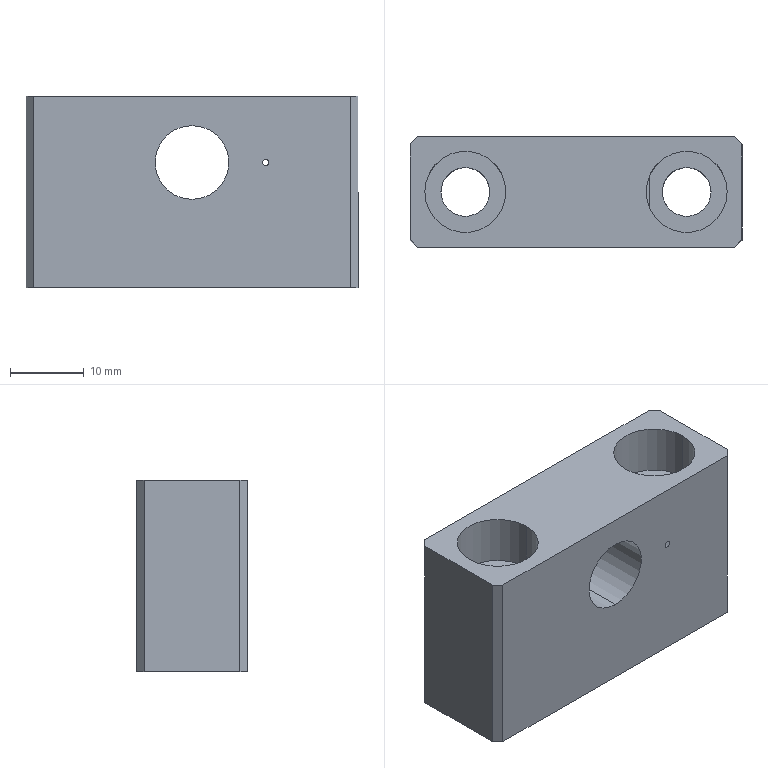Part | SolidWorks | features HoleWzd 3, Chamfer 1, Cut 1, Extrusion 1 | 1 solid | 34 faces | box 45 x 15 x 26 mm | volume 12916 mm3 | cylinder 16 | plane 12 | cone 6 | commonest cylinder face diameters 6 x4 6.6 x4 11 x4 4.2 x2 10 x2
STEP:
#1=CARTESIAN_POINT('',(10.,1.,1.9));
#2=VERTEX_POINT('',#1);
#3=CARTESIAN_POINT('',(10.,1.,6.1));
#4=VERTEX_POINT('',#3);
#5=CARTESIAN_POINT('',(10.,1.,4.));
#6=DIRECTION('',(0.,1.,0.));
#7=DIRECTION('',(0.,0.,1.));
#8=AXIS2_PLACEMENT_3D('',#5,#6,#7);
#9=CIRCLE('',#8,2.1);
#10=EDGE_CURVE('',#2,#4,#9,.T.);
#11=ORIENTED_EDGE('',*,*,#10,.F.);
#12=CARTESIAN_POINT('',(10.,15.,1.9));
#13=VERTEX_POINT('',#12);
#14=CARTESIAN_POINT('',(10.,15.,1.9));
#15=DIRECTION('',(0.,1.,0.));
#16=VECTOR('',#15,1000.);
#17=LINE('',#14,#16);
#18=EDGE_CURVE('',#2,#13,#17,.T.);
#19=ORIENTED_EDGE('',*,*,#18,.T.);
#20=CARTESIAN_POINT('',(10.,15.,6.1));
#21=VERTEX_POINT('',#20);
#22=CARTESIAN_POINT('',(10.,15.,4.));
#23=DIRECTION('',(0.,1.,0.));
#24=DIRECTION('',(0.,0.,1.));
#25=AXIS2_PLACEMENT_3D('',#22,#23,#24);
#26=CIRCLE('',#25,2.1);
#27=EDGE_CURVE('',#13,#21,#26,.T.);
#28=ORIENTED_EDGE('',*,*,#27,.T.);
#29=CARTESIAN_POINT('',(10.,15.,6.1));
#30=DIRECTION('',(0.,1.,0.));
#31=VECTOR('',#30,1000.);
#32=LINE('',#29,#31);
#33=EDGE_CURVE('',#4,#21,#32,.T.);
#34=ORIENTED_EDGE('',*,*,#33,.F.);
#35=EDGE_LOOP('',(#11,#19,#28,#34));
#36=FACE_OUTER_BOUND('',#35,.T.);
#37=CARTESIAN_POINT('',(10.,15.,4.));
#38=DIRECTION('',(0.,1.,0.));
#39=DIRECTION('',(0.,0.,1.));
#40=AXIS2_PLACEMENT_3D('',#37,#38,#39);
#41=CYLINDRICAL_SURFACE('',#40,2.1);
#42=ADVANCED_FACE('',(#36),#41,.F.);
#43=CARTESIAN_POINT('',(10.,0.,3.564));
#44=VERTEX_POINT('',#43);
#45=CARTESIAN_POINT('',(10.,0.,4.436));
#46=VERTEX_POINT('',#45);
#47=CARTESIAN_POINT('',(10.,0.,4.));
#48=DIRECTION('',(0.,1.,0.));
#49=DIRECTION('',(0.,0.,1.));
#50=AXIS2_PLACEMENT_3D('',#47,#48,#49);
#51=CIRCLE('',#50,0.4357);
#52=EDGE_CURVE('',#44,#46,#51,.T.);
#53=ORIENTED_EDGE('',*,*,#52,.F.);
#54=CARTESIAN_POINT('',(10.,1.,1.9));
#55=DIRECTION('',(0.,0.515,-0.8572));
#56=VECTOR('',#55,1000.);
#57=LINE('',#54,#56);
#58=EDGE_CURVE('',#44,#2,#57,.T.);
#59=ORIENTED_EDGE('',*,*,#58,.T.);
#60=ORIENTED_EDGE('',*,*,#10,.T.);
#61=CARTESIAN_POINT('',(10.,1.,6.1));
#62=DIRECTION('',(0.,0.515,0.8572));
#63=VECTOR('',#62,1000.);
#64=LINE('',#61,#63);
#65=EDGE_CURVE('',#46,#4,#64,.T.);
#66=ORIENTED_EDGE('',*,*,#65,.F.);
#67=EDGE_LOOP('',(#53,#59,#60,#66));
#68=FACE_OUTER_BOUND('',#67,.T.);
#69=CARTESIAN_POINT('',(10.,1.,4.));
#70=DIRECTION('',(0.,1.,0.));
#71=DIRECTION('',(0.,0.,1.));
#72=AXIS2_PLACEMENT_3D('',#69,#70,#71);
#73=CONICAL_SURFACE('',#72,2.1,1.03);
#74=ADVANCED_FACE('',(#68),#73,.F.);
#75=CARTESIAN_POINT('',(9.5,7.5,6.2));
#76=VERTEX_POINT('',#75);
#77=CARTESIAN_POINT('',(20.5,7.5,6.2));
#78=VERTEX_POINT('',#77);
#79=CARTESIAN_POINT('',(15.,7.5,6.2));
#80=DIRECTION('',(0.,0.,1.));
#81=DIRECTION('',(1.,0.,0.));
#82=AXIS2_PLACEMENT_3D('',#79,#80,#81);
#83=CIRCLE('',#82,5.5);
#84=EDGE_CURVE('',#76,#78,#83,.T.);
#85=ORIENTED_EDGE('',*,*,#84,.F.);
#86=CARTESIAN_POINT('',(9.5,7.5,13.));
#87=VERTEX_POINT('',#86);
#88=CARTESIAN_POINT('',(9.5,7.5,13.));
#89=DIRECTION('',(0.,0.,1.));
#90=VECTOR('',#89,1000.);
#91=LINE('',#88,#90);
#92=EDGE_CURVE('',#76,#87,#91,.T.);
#93=ORIENTED_EDGE('',*,*,#92,.T.);
#94=CARTESIAN_POINT('',(20.5,7.5,13.));
#95=VERTEX_POINT('',#94);
#96=CARTESIAN_POINT('',(15.,7.5,13.));
#97=DIRECTION('',(0.,0.,1.));
#98=DIRECTION('',(1.,0.,0.));
#99=AXIS2_PLACEMENT_3D('',#96,#97,#98);
#100=CIRCLE('',#99,5.5);
#101=EDGE_CURVE('',#87,#95,#100,.T.);
#102=ORIENTED_EDGE('',*,*,#101,.T.);
#103=CARTESIAN_POINT('',(20.5,7.5,13.));
#104=DIRECTION('',(0.,0.,1.));
#105=VECTOR('',#104,1000.);
#106=LINE('',#103,#105);
#107=EDGE_CURVE('',#78,#95,#106,.T.);
#108=ORIENTED_EDGE('',*,*,#107,.F.);
#109=EDGE_LOOP('',(#85,#93,#102,#108));
#110=FACE_OUTER_BOUND('',#109,.T.);
#111=CARTESIAN_POINT('',(15.,7.5,13.));
#112=DIRECTION('',(0.,0.,1.));
#113=DIRECTION('',(1.,0.,0.));
#114=AXIS2_PLACEMENT_3D('',#111,#112,#113);
#115=CYLINDRICAL_SURFACE('',#114,5.5);
#116=ADVANCED_FACE('',(#110),#115,.F.);
#117=CARTESIAN_POINT('',(11.7,7.5,-13.));
#118=VERTEX_POINT('',#117);
#119=CARTESIAN_POINT('',(18.3,7.5,-13.));
#120=VERTEX_POINT('',#119);
#121=CARTESIAN_POINT('',(15.,7.5,-13.));
#122=DIRECTION('',(0.,0.,1.));
#123=DIRECTION('',(1.,0.,0.));
#124=AXIS2_PLACEMENT_3D('',#121,#122,#123);
#125=CIRCLE('',#124,3.3);
#126=EDGE_CURVE('',#118,#120,#125,.T.);
#127=ORIENTED_EDGE('',*,*,#126,.F.);
#128=CARTESIAN_POINT('',(11.7,7.5,2.767));
#129=VERTEX_POINT('',#128);
#130=CARTESIAN_POINT('',(11.7,7.5,13.));
#131=DIRECTION('',(0.,0.,1.));
#132=VECTOR('',#131,1000.);
#133=LINE('',#130,#132);
#134=EDGE_CURVE('',#118,#129,#133,.T.);
#135=ORIENTED_EDGE('',*,*,#134,.T.);
#136=CARTESIAN_POINT('',(11.7,7.5,5.233));
#137=VERTEX_POINT('',#136);
#138=CARTESIAN_POINT('',(11.7,7.5,2.767));
#139=CARTESIAN_POINT('',(11.7,7.309,2.767));
#140=CARTESIAN_POINT('',(11.716,7.122,2.789));
#141=CARTESIAN_POINT('',(11.779,6.758,2.883));
#142=CARTESIAN_POINT('',(11.824,6.589,2.954));
#143=CARTESIAN_POINT('',(11.902,6.361,3.108));
#144=CARTESIAN_POINT('',(11.929,6.29,3.167));
#145=CARTESIAN_POINT('',(11.981,6.166,3.3));
#146=CARTESIAN_POINT('',(12.006,6.11,3.375));
#147=CARTESIAN_POINT('',(12.071,5.976,3.617));
#148=CARTESIAN_POINT('',(12.1,5.926,3.805));
#149=CARTESIAN_POINT('',(12.1,5.924,4.184));
#150=CARTESIAN_POINT('',(12.073,5.973,4.376));
#151=CARTESIAN_POINT('',(11.987,6.151,4.701));
#152=CARTESIAN_POINT('',(11.93,6.279,4.836));
#153=CARTESIAN_POINT('',(11.826,6.583,5.044));
#154=CARTESIAN_POINT('',(11.78,6.756,5.116));
#155=CARTESIAN_POINT('',(11.717,7.12,5.211));
#156=CARTESIAN_POINT('',(11.7,7.31,5.233));
#157=CARTESIAN_POINT('',(11.7,7.5,5.233));
#158=B_SPLINE_CURVE_WITH_KNOTS('',3,(#138,#139,#140,#141,#142,#143,#144,#145,#146,#147,#148,#149,#150,#151,#152,#153,#154,#155,#156,#157),.UNSPECIFIED.,.F.,.F.,(4,2,2,2,2,2,2,2,2,4),(0.,0.0005661,0.001132,0.001415,0.001698,0.002264,0.002831,0.003397,0.003963,0.004529),.UNSPECIFIED.);
#159=EDGE_CURVE('',#129,#137,#158,.T.);
#160=ORIENTED_EDGE('',*,*,#159,.T.);
#161=CARTESIAN_POINT('',(11.7,7.5,6.2));
#162=VERTEX_POINT('',#161);
#163=CARTESIAN_POINT('',(11.7,7.5,13.));
#164=DIRECTION('',(0.,0.,1.));
#165=VECTOR('',#164,1000.);
#166=LINE('',#163,#165);
#167=EDGE_CURVE('',#137,#162,#166,.T.);
#168=ORIENTED_EDGE('',*,*,#167,.T.);
#169=CARTESIAN_POINT('',(18.3,7.5,6.2));
#170=VERTEX_POINT('',#169);
#171=CARTESIAN_POINT('',(15.,7.5,6.2));
#172=DIRECTION('',(0.,0.,1.));
#173=DIRECTION('',(1.,0.,0.));
#174=AXIS2_PLACEMENT_3D('',#171,#172,#173);
#175=CIRCLE('',#174,3.3);
#176=EDGE_CURVE('',#162,#170,#175,.T.);
#177=ORIENTED_EDGE('',*,*,#176,.T.);
#178=CARTESIAN_POINT('',(18.3,7.5,13.));
#179=DIRECTION('',(0.,0.,1.));
#180=VECTOR('',#179,1000.);
#181=LINE('',#178,#180);
#182=EDGE_CURVE('',#120,#170,#181,.T.);
#183=ORIENTED_EDGE('',*,*,#182,.F.);
#184=EDGE_LOOP('',(#127,#135,#160,#168,#177,#183));
#185=FACE_OUTER_BOUND('',#184,.T.);
#186=CARTESIAN_POINT('',(15.,7.5,13.));
#187=DIRECTION('',(0.,0.,1.));
#188=DIRECTION('',(1.,0.,0.));
#189=AXIS2_PLACEMENT_3D('',#186,#187,#188);
#190=CYLINDRICAL_SURFACE('',#189,3.3);
#191=ADVANCED_FACE('',(#185),#190,.F.);
#192=CARTESIAN_POINT('',(-20.5,7.5,6.2));
#193=VERTEX_POINT('',#192);
#194=CARTESIAN_POINT('',(-9.5,7.5,6.2));
#195=VERTEX_POINT('',#194);
#196=CARTESIAN_POINT('',(-15.,7.5,6.2));
#197=DIRECTION('',(0.,0.,1.));
#198=DIRECTION('',(1.,0.,0.));
#199=AXIS2_PLACEMENT_3D('',#196,#197,#198);
#200=CIRCLE('',#199,5.5);
#201=EDGE_CURVE('',#193,#195,#200,.T.);
#202=ORIENTED_EDGE('',*,*,#201,.F.);
#203=CARTESIAN_POINT('',(-20.5,7.5,13.));
#204=VERTEX_POINT('',#203);
#205=CARTESIAN_POINT('',(-20.5,7.5,13.));
#206=DIRECTION('',(0.,0.,1.));
#207=VECTOR('',#206,1000.);
#208=LINE('',#205,#207);
#209=EDGE_CURVE('',#193,#204,#208,.T.);
#210=ORIENTED_EDGE('',*,*,#209,.T.);
#211=CARTESIAN_POINT('',(-9.5,7.5,13.));
#212=VERTEX_POINT('',#211);
#213=CARTESIAN_POINT('',(-15.,7.5,13.));
#214=DIRECTION('',(0.,0.,1.));
#215=DIRECTION('',(1.,0.,0.));
#216=AXIS2_PLACEMENT_3D('',#213,#214,#215);
#217=CIRCLE('',#216,5.5);
#218=EDGE_CURVE('',#204,#212,#217,.T.);
#219=ORIENTED_EDGE('',*,*,#218,.T.);
#220=CARTESIAN_POINT('',(-9.5,7.5,13.));
#221=DIRECTION('',(0.,0.,1.));
#222=VECTOR('',#221,1000.);
#223=LINE('',#220,#222);
#224=EDGE_CURVE('',#195,#212,#223,.T.);
#225=ORIENTED_EDGE('',*,*,#224,.F.);
#226=EDGE_LOOP('',(#202,#210,#219,#225));
#227=FACE_OUTER_BOUND('',#226,.T.);
#228=CARTESIAN_POINT('',(-15.,7.5,13.));
#229=DIRECTION('',(0.,0.,1.));
#230=DIRECTION('',(1.,0.,0.));
#231=AXIS2_PLACEMENT_3D('',#228,#229,#230);
#232=CYLINDRICAL_SURFACE('',#231,5.5);
#233=ADVANCED_FACE('',(#227),#232,.F.);
#234=CARTESIAN_POINT('',(-18.3,7.5,-13.));
#235=VERTEX_POINT('',#234);
#236=CARTESIAN_POINT('',(-11.7,7.5,-13.));
#237=VERTEX_POINT('',#236);
#238=CARTESIAN_POINT('',(-15.,7.5,-13.));
#239=DIRECTION('',(0.,0.,1.));
#240=DIRECTION('',(1.,0.,0.));
#241=AXIS2_PLACEMENT_3D('',#238,#239,#240);
#242=CIRCLE('',#241,3.3);
#243=EDGE_CURVE('',#235,#237,#242,.T.);
#244=ORIENTED_EDGE('',*,*,#243,.F.);
#245=CARTESIAN_POINT('',(-18.3,7.5,6.2));
#246=VERTEX_POINT('',#245);
#247=CARTESIAN_POINT('',(-18.3,7.5,13.));
#248=DIRECTION('',(0.,0.,1.));
#249=VECTOR('',#248,1000.);
#250=LINE('',#247,#249);
#251=EDGE_CURVE('',#235,#246,#250,.T.);
#252=ORIENTED_EDGE('',*,*,#251,.T.);
#253=CARTESIAN_POINT('',(-11.7,7.5,6.2));
#254=VERTEX_POINT('',#253);
#255=CARTESIAN_POINT('',(-15.,7.5,6.2));
#256=DIRECTION('',(0.,0.,1.));
#257=DIRECTION('',(1.,0.,0.));
#258=AXIS2_PLACEMENT_3D('',#255,#256,#257);
#259=CIRCLE('',#258,3.3);
#260=EDGE_CURVE('',#246,#254,#259,.T.);
#261=ORIENTED_EDGE('',*,*,#260,.T.);
#262=CARTESIAN_POINT('',(-11.7,7.5,13.));
#263=DIRECTION('',(0.,0.,1.));
#264=VECTOR('',#263,1000.);
#265=LINE('',#262,#264);
#266=EDGE_CURVE('',#237,#254,#265,.T.);
#267=ORIENTED_EDGE('',*,*,#266,.F.);
#268=EDGE_LOOP('',(#244,#252,#261,#267));
#269=FACE_OUTER_BOUND('',#268,.T.);
#270=CARTESIAN_POINT('',(-15.,7.5,13.));
#271=DIRECTION('',(0.,0.,1.));
#272=DIRECTION('',(1.,0.,0.));
#273=AXIS2_PLACEMENT_3D('',#270,#271,#272);
#274=CYLINDRICAL_SURFACE('',#273,3.3);
#275=ADVANCED_FACE('',(#269),#274,.F.);
#276=CARTESIAN_POINT('',(-2.,7.5,-3.));
#277=VERTEX_POINT('',#276);
#278=CARTESIAN_POINT('',(-8.,7.5,-3.));
#279=VERTEX_POINT('',#278);
#280=CARTESIAN_POINT('',(-5.,7.5,-3.));
#281=DIRECTION('',(0.,0.,-1.));
#282=DIRECTION('',(-1.,0.,0.));
#283=AXIS2_PLACEMENT_3D('',#280,#281,#282);
#284=CIRCLE('',#283,3.);
#285=EDGE_CURVE('',#277,#279,#284,.T.);
#286=ORIENTED_EDGE('',*,*,#285,.F.);
#287=CARTESIAN_POINT('',(-2.,7.5,-13.));
#288=VERTEX_POINT('',#287);
#289=CARTESIAN_POINT('',(-2.,7.5,-13.));
#290=DIRECTION('',(0.,0.,-1.));
#291=VECTOR('',#290,1000.);
#292=LINE('',#289,#291);
#293=EDGE_CURVE('',#277,#288,#292,.T.);
#294=ORIENTED_EDGE('',*,*,#293,.T.);
#295=CARTESIAN_POINT('',(-8.,7.5,-13.));
#296=VERTEX_POINT('',#295);
#297=CARTESIAN_POINT('',(-5.,7.5,-13.));
#298=DIRECTION('',(0.,0.,-1.));
#299=DIRECTION('',(-1.,0.,0.));
#300=AXIS2_PLACEMENT_3D('',#297,#298,#299);
#301=CIRCLE('',#300,3.);
#302=EDGE_CURVE('',#288,#296,#301,.T.);
#303=ORIENTED_EDGE('',*,*,#302,.T.);
#304=CARTESIAN_POINT('',(-8.,7.5,-13.));
#305=DIRECTION('',(0.,0.,-1.));
#306=VECTOR('',#305,1000.);
#307=LINE('',#304,#306);
#308=EDGE_CURVE('',#279,#296,#307,.T.);
#309=ORIENTED_EDGE('',*,*,#308,.F.);
#310=EDGE_LOOP('',(#286,#294,#303,#309));
#311=FACE_OUTER_BOUND('',#310,.T.);
#312=CARTESIAN_POINT('',(-5.,7.5,-13.));
#313=DIRECTION('',(0.,0.,-1.));
#314=DIRECTION('',(-1.,0.,0.));
#315=AXIS2_PLACEMENT_3D('',#312,#313,#314);
#316=CYLINDRICAL_SURFACE('',#315,3.);
#317=ADVANCED_FACE('',(#311),#316,.F.);
#318=CARTESIAN_POINT('',(-5.,7.5,-1.197));
#319=VERTEX_POINT('',#318);
#320=CARTESIAN_POINT('',(-8.,7.5,-3.));
#321=DIRECTION('',(-0.8572,0.,-0.515));
#322=VECTOR('',#321,1000.);
#323=LINE('',#320,#322);
#324=EDGE_CURVE('',#319,#279,#323,.T.);
#325=ORIENTED_EDGE('',*,*,#324,.F.);
#326=CARTESIAN_POINT('',(-2.,7.5,-3.));
#327=DIRECTION('',(0.8572,0.,-0.515));
#328=VECTOR('',#327,1000.);
#329=LINE('',#326,#328);
#330=EDGE_CURVE('',#319,#277,#329,.T.);
#331=ORIENTED_EDGE('',*,*,#330,.T.);
#332=ORIENTED_EDGE('',*,*,#285,.T.);
#333=EDGE_LOOP('',(#325,#331,#332));
#334=FACE_OUTER_BOUND('',#333,.T.);
#335=CARTESIAN_POINT('',(-5.,7.5,-3.));
#336=DIRECTION('',(0.,0.,-1.));
#337=DIRECTION('',(-1.,0.,0.));
#338=AXIS2_PLACEMENT_3D('',#335,#336,#337);
#339=CONICAL_SURFACE('',#338,3.,1.03);
#340=ADVANCED_FACE('',(#334),#339,.F.);
#341=CARTESIAN_POINT('',(8.,7.5,-3.));
#342=VERTEX_POINT('',#341);
#343=CARTESIAN_POINT('',(2.,7.5,-3.));
#344=VERTEX_POINT('',#343);
#345=CARTESIAN_POINT('',(5.,7.5,-3.));
#346=DIRECTION('',(0.,0.,-1.));
#347=DIRECTION('',(-1.,0.,0.));
#348=AXIS2_PLACEMENT_3D('',#345,#346,#347);
#349=CIRCLE('',#348,3.);
#350=EDGE_CURVE('',#342,#344,#349,.T.);
#351=ORIENTED_EDGE('',*,*,#350,.F.);
#352=CARTESIAN_POINT('',(8.,7.5,-13.));
#353=VERTEX_POINT('',#352);
#354=CARTESIAN_POINT('',(8.,7.5,-13.));
#355=DIRECTION('',(0.,0.,-1.));
#356=VECTOR('',#355,1000.);
#357=LINE('',#354,#356);
#358=EDGE_CURVE('',#342,#353,#357,.T.);
#359=ORIENTED_EDGE('',*,*,#358,.T.);
#360=CARTESIAN_POINT('',(2.,7.5,-13.));
#361=VERTEX_POINT('',#360);
#362=CARTESIAN_POINT('',(5.,7.5,-13.));
#363=DIRECTION('',(0.,0.,-1.));
#364=DIRECTION('',(-1.,0.,0.));
#365=AXIS2_PLACEMENT_3D('',#362,#363,#364);
#366=CIRCLE('',#365,3.);
#367=EDGE_CURVE('',#353,#361,#366,.T.);
#368=ORIENTED_EDGE('',*,*,#367,.T.);
#369=CARTESIAN_POINT('',(2.,7.5,-13.));
#370=DIRECTION('',(0.,0.,-1.));
#371=VECTOR('',#370,1000.);
#372=LINE('',#369,#371);
#373=EDGE_CURVE('',#344,#361,#372,.T.);
#374=ORIENTED_EDGE('',*,*,#373,.F.);
#375=EDGE_LOOP('',(#351,#359,#368,#374));
#376=FACE_OUTER_BOUND('',#375,.T.);
#377=CARTESIAN_POINT('',(5.,7.5,-13.));
#378=DIRECTION('',(0.,0.,-1.));
#379=DIRECTION('',(-1.,0.,0.));
#380=AXIS2_PLACEMENT_3D('',#377,#378,#379);
#381=CYLINDRICAL_SURFACE('',#380,3.);
#382=ADVANCED_FACE('',(#376),#381,.F.);
#383=CARTESIAN_POINT('',(5.,7.5,-1.197));
#384=VERTEX_POINT('',#383);
#385=CARTESIAN_POINT('',(2.,7.5,-3.));
#386=DIRECTION('',(-0.8572,0.,-0.515));
#387=VECTOR('',#386,1000.);
#388=LINE('',#385,#387);
#389=EDGE_CURVE('',#384,#344,#388,.T.);
#390=ORIENTED_EDGE('',*,*,#389,.F.);
#391=CARTESIAN_POINT('',(8.,7.5,-3.));
#392=DIRECTION('',(0.8572,0.,-0.515));
#393=VECTOR('',#392,1000.);
#394=LINE('',#391,#393);
#395=EDGE_CURVE('',#384,#342,#394,.T.);
#396=ORIENTED_EDGE('',*,*,#395,.T.);
#397=ORIENTED_EDGE('',*,*,#350,.T.);
#398=EDGE_LOOP('',(#390,#396,#397));
#399=FACE_OUTER_BOUND('',#398,.T.);
#400=CARTESIAN_POINT('',(5.,7.5,-3.));
#401=DIRECTION('',(0.,0.,-1.));
#402=DIRECTION('',(-1.,0.,0.));
#403=AXIS2_PLACEMENT_3D('',#400,#401,#402);
#404=CONICAL_SURFACE('',#403,3.,1.03);
#405=ADVANCED_FACE('',(#399),#404,.F.);
#406=CARTESIAN_POINT('',(0.,0.,-1.));
#407=VERTEX_POINT('',#406);
#408=CARTESIAN_POINT('',(0.,0.,9.));
#409=VERTEX_POINT('',#408);
#410=CARTESIAN_POINT('',(0.,0.,4.));
#411=DIRECTION('',(0.,1.,0.));
#412=DIRECTION('',(0.,0.,1.));
#413=AXIS2_PLACEMENT_3D('',#410,#411,#412);
#414=CIRCLE('',#413,5.);
#415=EDGE_CURVE('',#407,#409,#414,.T.);
#416=ORIENTED_EDGE('',*,*,#415,.F.);
#417=CARTESIAN_POINT('',(0.,15.,-1.));
#418=VERTEX_POINT('',#417);
#419=CARTESIAN_POINT('',(0.,0.,-1.));
#420=DIRECTION('',(0.,1.,0.));
#421=VECTOR('',#420,1000.);
#422=LINE('',#419,#421);
#423=EDGE_CURVE('',#407,#418,#422,.T.);
#424=ORIENTED_EDGE('',*,*,#423,.T.);
#425=CARTESIAN_POINT('',(0.,15.,9.));
#426=VERTEX_POINT('',#425);
#427=CARTESIAN_POINT('',(0.,15.,4.));
#428=DIRECTION('',(0.,1.,0.));
#429=DIRECTION('',(0.,0.,1.));
#430=AXIS2_PLACEMENT_3D('',#427,#428,#429);
#431=CIRCLE('',#430,5.);
#432=EDGE_CURVE('',#418,#426,#431,.T.);
#433=ORIENTED_EDGE('',*,*,#432,.T.);
#434=CARTESIAN_POINT('',(0.,0.,9.));
#435=DIRECTION('',(0.,1.,0.));
#436=VECTOR('',#435,1000.);
#437=LINE('',#434,#436);
#438=EDGE_CURVE('',#409,#426,#437,.T.);
#439=ORIENTED_EDGE('',*,*,#438,.F.);
#440=EDGE_LOOP('',(#416,#424,#433,#439));
#441=FACE_OUTER_BOUND('',#440,.T.);
#442=CARTESIAN_POINT('',(0.,0.,4.));
#443=DIRECTION('',(0.,1.,0.));
#444=DIRECTION('',(0.,0.,1.));
#445=AXIS2_PLACEMENT_3D('',#442,#443,#444);
#446=CYLINDRICAL_SURFACE('',#445,5.);
#447=ADVANCED_FACE('',(#441),#446,.F.);
#448=CARTESIAN_POINT('',(-15.,7.5,13.));
#449=DIRECTION('',(0.,0.,1.));
#450=DIRECTION('',(1.,0.,0.));
#451=AXIS2_PLACEMENT_3D('',#448,#449,#450);
#452=CIRCLE('',#451,5.5);
#453=EDGE_CURVE('',#212,#204,#452,.T.);
#454=ORIENTED_EDGE('',*,*,#453,.F.);
#455=ORIENTED_EDGE('',*,*,#218,.F.);
#456=EDGE_LOOP('',(#454,#455));
#457=FACE_BOUND('',#456,.T.);
#458=CARTESIAN_POINT('',(-21.5,0.,13.));
#459=VERTEX_POINT('',#458);
#460=CARTESIAN_POINT('',(21.5,0.,13.));
#461=VERTEX_POINT('',#460);
#462=CARTESIAN_POINT('',(-22.5,0.,13.));
#463=DIRECTION('',(1.,0.,0.));
#464=VECTOR('',#463,1000.);
#465=LINE('',#462,#464);
#466=EDGE_CURVE('',#459,#461,#465,.T.);
#467=ORIENTED_EDGE('',*,*,#466,.T.);
#468=CARTESIAN_POINT('',(22.5,1.,13.));
#469=VERTEX_POINT('',#468);
#470=CARTESIAN_POINT('',(22.5,1.,13.));
#471=DIRECTION('',(0.7071,0.7071,0.));
#472=VECTOR('',#471,1000.);
#473=LINE('',#470,#472);
#474=EDGE_CURVE('',#461,#469,#473,.T.);
#475=ORIENTED_EDGE('',*,*,#474,.T.);
#476=CARTESIAN_POINT('',(22.5,14.,13.));
#477=VERTEX_POINT('',#476);
#478=CARTESIAN_POINT('',(22.5,15.,13.));
#479=DIRECTION('',(0.,-1.,0.));
#480=VECTOR('',#479,1000.);
#481=LINE('',#478,#480);
#482=EDGE_CURVE('',#477,#469,#481,.T.);
#483=ORIENTED_EDGE('',*,*,#482,.F.);
#484=CARTESIAN_POINT('',(21.5,15.,13.));
#485=VERTEX_POINT('',#484);
#486=CARTESIAN_POINT('',(21.5,15.,13.));
#487=DIRECTION('',(-0.7071,0.7071,0.));
#488=VECTOR('',#487,1000.);
#489=LINE('',#486,#488);
#490=EDGE_CURVE('',#477,#485,#489,.T.);
#491=ORIENTED_EDGE('',*,*,#490,.T.);
#492=CARTESIAN_POINT('',(-21.5,15.,13.));
#493=VERTEX_POINT('',#492);
#494=CARTESIAN_POINT('',(-22.5,15.,13.));
#495=DIRECTION('',(1.,0.,0.));
#496=VECTOR('',#495,1000.);
#497=LINE('',#494,#496);
#498=EDGE_CURVE('',#493,#485,#497,.T.);
#499=ORIENTED_EDGE('',*,*,#498,.F.);
#500=CARTESIAN_POINT('',(-22.5,14.,13.));
#501=VERTEX_POINT('',#500);
#502=CARTESIAN_POINT('',(-21.5,15.,13.));
#503=DIRECTION('',(-0.7071,-0.7071,0.));
#504=VECTOR('',#503,1000.);
#505=LINE('',#502,#504);
#506=EDGE_CURVE('',#493,#501,#505,.T.);
#507=ORIENTED_EDGE('',*,*,#506,.T.);
#508=CARTESIAN_POINT('',(-22.5,1.,13.));
#509=VERTEX_POINT('',#508);
#510=CARTESIAN_POINT('',(-22.5,15.,13.));
#511=DIRECTION('',(0.,-1.,0.));
#512=VECTOR('',#511,1000.);
#513=LINE('',#510,#512);
#514=EDGE_CURVE('',#501,#509,#513,.T.);
#515=ORIENTED_EDGE('',*,*,#514,.T.);
#516=CARTESIAN_POINT('',(-22.5,1.,13.));
#517=DIRECTION('',(0.7071,-0.7071,0.));
#518=VECTOR('',#517,1000.);
#519=LINE('',#516,#518);
#520=EDGE_CURVE('',#509,#459,#519,.T.);
#521=ORIENTED_EDGE('',*,*,#520,.T.);
#522=EDGE_LOOP('',(#467,#475,#483,#491,#499,#507,#515,#521));
#523=FACE_OUTER_BOUND('',#522,.T.);
#524=CARTESIAN_POINT('',(15.,7.5,13.));
#525=DIRECTION('',(0.,0.,1.));
#526=DIRECTION('',(1.,0.,0.));
#527=AXIS2_PLACEMENT_3D('',#524,#525,#526);
#528=CIRCLE('',#527,5.5);
#529=EDGE_CURVE('',#95,#87,#528,.T.);
#530=ORIENTED_EDGE('',*,*,#529,.F.);
#531=ORIENTED_EDGE('',*,*,#101,.F.);
#532=EDGE_LOOP('',(#530,#531));
#533=FACE_BOUND('',#532,.T.);
#534=CARTESIAN_POINT('',(-22.5,15.,13.));
#535=DIRECTION('',(0.,0.,-1.));
#536=DIRECTION('',(-1.,0.,0.));
#537=AXIS2_PLACEMENT_3D('',#534,#535,#536);
#538=PLANE('',#537);
#539=ADVANCED_FACE('',(#457,#523,#533),#538,.F.);
#540=ORIENTED_EDGE('',*,*,#482,.T.);
#541=CARTESIAN_POINT('',(22.5,1.,-13.));
#542=VERTEX_POINT('',#541);
#543=CARTESIAN_POINT('',(22.5,1.,-13.));
#544=DIRECTION('',(0.,0.,-1.));
#545=VECTOR('',#544,1000.);
#546=LINE('',#543,#545);
#547=EDGE_CURVE('',#469,#542,#546,.T.);
#548=ORIENTED_EDGE('',*,*,#547,.T.);
#549=CARTESIAN_POINT('',(22.5,14.,-13.));
#550=VERTEX_POINT('',#549);
#551=CARTESIAN_POINT('',(22.5,15.,-13.));
#552=DIRECTION('',(0.,-1.,0.));
#553=VECTOR('',#552,1000.);
#554=LINE('',#551,#553);
#555=EDGE_CURVE('',#550,#542,#554,.T.);
#556=ORIENTED_EDGE('',*,*,#555,.F.);
#557=CARTESIAN_POINT('',(22.5,14.,13.));
#558=DIRECTION('',(0.,0.,1.));
#559=VECTOR('',#558,1000.);
#560=LINE('',#557,#559);
#561=EDGE_CURVE('',#550,#477,#560,.T.);
#562=ORIENTED_EDGE('',*,*,#561,.T.);
#563=EDGE_LOOP('',(#540,#548,#556,#562));
#564=FACE_OUTER_BOUND('',#563,.T.);
#565=CARTESIAN_POINT('',(22.5,15.,-13.));
#566=DIRECTION('',(-1.,0.,0.));
#567=DIRECTION('',(0.,0.,1.));
#568=AXIS2_PLACEMENT_3D('',#565,#566,#567);
#569=PLANE('',#568);
#570=ADVANCED_FACE('',(#564),#569,.F.);
#571=CARTESIAN_POINT('',(15.,7.5,-13.));
#572=DIRECTION('',(0.,0.,1.));
#573=DIRECTION('',(1.,0.,0.));
#574=AXIS2_PLACEMENT_3D('',#571,#572,#573);
#575=CIRCLE('',#574,3.3);
#576=EDGE_CURVE('',#120,#118,#575,.T.);
#577=ORIENTED_EDGE('',*,*,#576,.T.);
#578=ORIENTED_EDGE('',*,*,#126,.T.);
#579=EDGE_LOOP('',(#577,#578));
#580=FACE_BOUND('',#579,.T.);
#581=CARTESIAN_POINT('',(-15.,7.5,-13.));
#582=DIRECTION('',(0.,0.,1.));
#583=DIRECTION('',(1.,0.,0.));
#584=AXIS2_PLACEMENT_3D('',#581,#582,#583);
#585=CIRCLE('',#584,3.3);
#586=EDGE_CURVE('',#237,#235,#585,.T.);
#587=ORIENTED_EDGE('',*,*,#586,.T.);
#588=ORIENTED_EDGE('',*,*,#243,.T.);
#589=EDGE_LOOP('',(#587,#588));
#590=FACE_BOUND('',#589,.T.);
#591=CARTESIAN_POINT('',(-5.,7.5,-13.));
#592=DIRECTION('',(0.,0.,-1.));
#593=DIRECTION('',(-1.,0.,0.));
#594=AXIS2_PLACEMENT_3D('',#591,#592,#593);
#595=CIRCLE('',#594,3.);
#596=EDGE_CURVE('',#296,#288,#595,.T.);
#597=ORIENTED_EDGE('',*,*,#596,.F.);
#598=ORIENTED_EDGE('',*,*,#302,.F.);
#599=EDGE_LOOP('',(#597,#598));
#600=FACE_BOUND('',#599,.T.);
#601=CARTESIAN_POINT('',(5.,7.5,-13.));
#602=DIRECTION('',(0.,0.,-1.));
#603=DIRECTION('',(-1.,0.,0.));
#604=AXIS2_PLACEMENT_3D('',#601,#602,#603);
#605=CIRCLE('',#604,3.);
#606=EDGE_CURVE('',#361,#353,#605,.T.);
#607=ORIENTED_EDGE('',*,*,#606,.F.);
#608=ORIENTED_EDGE('',*,*,#367,.F.);
#609=EDGE_LOOP('',(#607,#608));
#610=FACE_BOUND('',#609,.T.);
#611=ORIENTED_EDGE('',*,*,#555,.T.);
#612=CARTESIAN_POINT('',(21.5,0.,-13.));
#613=VERTEX_POINT('',#612);
#614=CARTESIAN_POINT('',(22.5,1.,-13.));
#615=DIRECTION('',(-0.7071,-0.7071,0.));
#616=VECTOR('',#615,1000.);
#617=LINE('',#614,#616);
#618=EDGE_CURVE('',#542,#613,#617,.T.);
#619=ORIENTED_EDGE('',*,*,#618,.T.);
#620=CARTESIAN_POINT('',(-21.5,0.,-13.));
#621=VERTEX_POINT('',#620);
#622=CARTESIAN_POINT('',(-22.5,0.,-13.));
#623=DIRECTION('',(-1.,0.,0.));
#624=VECTOR('',#623,1000.);
#625=LINE('',#622,#624);
#626=EDGE_CURVE('',#613,#621,#625,.T.);
#627=ORIENTED_EDGE('',*,*,#626,.T.);
#628=CARTESIAN_POINT('',(-22.5,1.,-13.));
#629=VERTEX_POINT('',#628);
#630=CARTESIAN_POINT('',(-22.5,1.,-13.));
#631=DIRECTION('',(-0.7071,0.7071,0.));
#632=VECTOR('',#631,1000.);
#633=LINE('',#630,#632);
#634=EDGE_CURVE('',#621,#629,#633,.T.);
#635=ORIENTED_EDGE('',*,*,#634,.T.);
#636=CARTESIAN_POINT('',(-22.5,14.,-13.));
#637=VERTEX_POINT('',#636);
#638=CARTESIAN_POINT('',(-22.5,15.,-13.));
#639=DIRECTION('',(0.,-1.,0.));
#640=VECTOR('',#639,1000.);
#641=LINE('',#638,#640);
#642=EDGE_CURVE('',#637,#629,#641,.T.);
#643=ORIENTED_EDGE('',*,*,#642,.F.);
#644=CARTESIAN_POINT('',(-21.5,15.,-13.));
#645=VERTEX_POINT('',#644);
#646=CARTESIAN_POINT('',(-21.5,15.,-13.));
#647=DIRECTION('',(0.7071,0.7071,0.));
#648=VECTOR('',#647,1000.);
#649=LINE('',#646,#648);
#650=EDGE_CURVE('',#637,#645,#649,.T.);
#651=ORIENTED_EDGE('',*,*,#650,.T.);
#652=CARTESIAN_POINT('',(21.5,15.,-13.));
#653=VERTEX_POINT('',#652);
#654=CARTESIAN_POINT('',(-22.5,15.,-13.));
#655=DIRECTION('',(-1.,0.,0.));
#656=VECTOR('',#655,1000.);
#657=LINE('',#654,#656);
#658=EDGE_CURVE('',#653,#645,#657,.T.);
#659=ORIENTED_EDGE('',*,*,#658,.F.);
#660=CARTESIAN_POINT('',(21.5,15.,-13.));
#661=DIRECTION('',(0.7071,-0.7071,0.));
#662=VECTOR('',#661,1000.);
#663=LINE('',#660,#662);
#664=EDGE_CURVE('',#653,#550,#663,.T.);
#665=ORIENTED_EDGE('',*,*,#664,.T.);
#666=EDGE_LOOP('',(#611,#619,#627,#635,#643,#651,#659,#665));
#667=FACE_OUTER_BOUND('',#666,.T.);
#668=CARTESIAN_POINT('',(-22.5,15.,-13.));
#669=DIRECTION('',(0.,0.,1.));
#670=DIRECTION('',(1.,0.,0.));
#671=AXIS2_PLACEMENT_3D('',#668,#669,#670);
#672=PLANE('',#671);
#673=ADVANCED_FACE('',(#580,#590,#600,#610,#667),#672,.F.);
#674=ORIENTED_EDGE('',*,*,#642,.T.);
#675=CARTESIAN_POINT('',(-22.5,1.,-13.));
#676=DIRECTION('',(0.,0.,1.));
#677=VECTOR('',#676,1000.);
#678=LINE('',#675,#677);
#679=EDGE_CURVE('',#629,#509,#678,.T.);
#680=ORIENTED_EDGE('',*,*,#679,.T.);
#681=ORIENTED_EDGE('',*,*,#514,.F.);
#682=CARTESIAN_POINT('',(-22.5,14.,-13.));
#683=DIRECTION('',(0.,0.,-1.));
#684=VECTOR('',#683,1000.);
#685=LINE('',#682,#684);
#686=EDGE_CURVE('',#501,#637,#685,.T.);
#687=ORIENTED_EDGE('',*,*,#686,.T.);
#688=EDGE_LOOP('',(#674,#680,#681,#687));
#689=FACE_OUTER_BOUND('',#688,.T.);
#690=CARTESIAN_POINT('',(-22.5,15.,-13.));
#691=DIRECTION('',(1.,0.,0.));
#692=DIRECTION('',(0.,0.,-1.));
#693=AXIS2_PLACEMENT_3D('',#690,#691,#692);
#694=PLANE('',#693);
#695=ADVANCED_FACE('',(#689),#694,.F.);
#696=CARTESIAN_POINT('',(10.,15.,4.));
#697=DIRECTION('',(0.,1.,0.));
#698=DIRECTION('',(0.,0.,1.));
#699=AXIS2_PLACEMENT_3D('',#696,#697,#698);
#700=CIRCLE('',#699,2.1);
#701=EDGE_CURVE('',#21,#13,#700,.T.);
#702=ORIENTED_EDGE('',*,*,#701,.F.);
#703=ORIENTED_EDGE('',*,*,#27,.F.);
#704=EDGE_LOOP('',(#702,#703));
#705=FACE_BOUND('',#704,.T.);
#706=CARTESIAN_POINT('',(0.,15.,4.));
#707=DIRECTION('',(0.,1.,0.));
#708=DIRECTION('',(0.,0.,1.));
#709=AXIS2_PLACEMENT_3D('',#706,#707,#708);
#710=CIRCLE('',#709,5.);
#711=EDGE_CURVE('',#426,#418,#710,.T.);
#712=ORIENTED_EDGE('',*,*,#711,.F.);
#713=ORIENTED_EDGE('',*,*,#432,.F.);
#714=EDGE_LOOP('',(#712,#713));
#715=FACE_BOUND('',#714,.T.);
#716=ORIENTED_EDGE('',*,*,#498,.T.);
#717=CARTESIAN_POINT('',(21.5,15.,-13.));
#718=DIRECTION('',(0.,0.,-1.));
#719=VECTOR('',#718,1000.);
#720=LINE('',#717,#719);
#721=EDGE_CURVE('',#485,#653,#720,.T.);
#722=ORIENTED_EDGE('',*,*,#721,.T.);
#723=ORIENTED_EDGE('',*,*,#658,.T.);
#724=CARTESIAN_POINT('',(-21.5,15.,13.));
#725=DIRECTION('',(0.,0.,1.));
#726=VECTOR('',#725,1000.);
#727=LINE('',#724,#726);
#728=EDGE_CURVE('',#645,#493,#727,.T.);
#729=ORIENTED_EDGE('',*,*,#728,.T.);
#730=EDGE_LOOP('',(#716,#722,#723,#729));
#731=FACE_OUTER_BOUND('',#730,.T.);
#732=CARTESIAN_POINT('',(22.5,15.,13.));
#733=DIRECTION('',(0.,1.,0.));
#734=DIRECTION('',(0.,0.,1.));
#735=AXIS2_PLACEMENT_3D('',#732,#733,#734);
#736=PLANE('',#735);
#737=ADVANCED_FACE('',(#705,#715,#731),#736,.T.);
#738=CARTESIAN_POINT('',(10.,0.,4.));
#739=DIRECTION('',(0.,1.,0.));
#740=DIRECTION('',(0.,0.,1.));
#741=AXIS2_PLACEMENT_3D('',#738,#739,#740);
#742=CIRCLE('',#741,0.4357);
#743=EDGE_CURVE('',#46,#44,#742,.T.);
#744=ORIENTED_EDGE('',*,*,#743,.T.);
#745=ORIENTED_EDGE('',*,*,#52,.T.);
#746=EDGE_LOOP('',(#744,#745));
#747=FACE_BOUND('',#746,.T.);
#748=CARTESIAN_POINT('',(0.,0.,4.));
#749=DIRECTION('',(0.,1.,0.));
#750=DIRECTION('',(0.,0.,1.));
#751=AXIS2_PLACEMENT_3D('',#748,#749,#750);
#752=CIRCLE('',#751,5.);
#753=EDGE_CURVE('',#409,#407,#752,.T.);
#754=ORIENTED_EDGE('',*,*,#753,.T.);
#755=ORIENTED_EDGE('',*,*,#415,.T.);
#756=EDGE_LOOP('',(#754,#755));
#757=FACE_BOUND('',#756,.T.);
#758=ORIENTED_EDGE('',*,*,#626,.F.);
#759=CARTESIAN_POINT('',(21.5,0.,13.));
#760=DIRECTION('',(0.,0.,1.));
#761=VECTOR('',#760,1000.);
#762=LINE('',#759,#761);
#763=EDGE_CURVE('',#613,#461,#762,.T.);
#764=ORIENTED_EDGE('',*,*,#763,.T.);
#765=ORIENTED_EDGE('',*,*,#466,.F.);
#766=CARTESIAN_POINT('',(-21.5,0.,13.));
#767=DIRECTION('',(0.,0.,-1.));
#768=VECTOR('',#767,1000.);
#769=LINE('',#766,#768);
#770=EDGE_CURVE('',#459,#621,#769,.T.);
#771=ORIENTED_EDGE('',*,*,#770,.T.);
#772=EDGE_LOOP('',(#758,#764,#765,#771));
#773=FACE_OUTER_BOUND('',#772,.T.);
#774=CARTESIAN_POINT('',(22.5,0.,13.));
#775=DIRECTION('',(0.,1.,0.));
#776=DIRECTION('',(0.,0.,1.));
#777=AXIS2_PLACEMENT_3D('',#774,#775,#776);
#778=PLANE('',#777);
#779=ADVANCED_FACE('',(#747,#757,#773),#778,.F.);
#780=ORIENTED_EDGE('',*,*,#423,.F.);
#781=ORIENTED_EDGE('',*,*,#753,.F.);
#782=ORIENTED_EDGE('',*,*,#438,.T.);
#783=ORIENTED_EDGE('',*,*,#711,.T.);
#784=EDGE_LOOP('',(#780,#781,#782,#783));
#785=FACE_OUTER_BOUND('',#784,.T.);
#786=CARTESIAN_POINT('',(0.,0.,4.));
#787=DIRECTION('',(0.,1.,0.));
#788=DIRECTION('',(0.,0.,1.));
#789=AXIS2_PLACEMENT_3D('',#786,#787,#788);
#790=CYLINDRICAL_SURFACE('',#789,5.);
#791=ADVANCED_FACE('',(#785),#790,.F.);
#792=ORIENTED_EDGE('',*,*,#395,.F.);
#793=ORIENTED_EDGE('',*,*,#389,.T.);
#794=CARTESIAN_POINT('',(5.,7.5,-3.));
#795=DIRECTION('',(0.,0.,-1.));
#796=DIRECTION('',(-1.,0.,0.));
#797=AXIS2_PLACEMENT_3D('',#794,#795,#796);
#798=CIRCLE('',#797,3.);
#799=EDGE_CURVE('',#344,#342,#798,.T.);
#800=ORIENTED_EDGE('',*,*,#799,.T.);
#801=EDGE_LOOP('',(#792,#793,#800));
#802=FACE_OUTER_BOUND('',#801,.T.);
#803=CARTESIAN_POINT('',(5.,7.5,-3.));
#804=DIRECTION('',(0.,0.,-1.));
#805=DIRECTION('',(-1.,0.,0.));
#806=AXIS2_PLACEMENT_3D('',#803,#804,#805);
#807=CONICAL_SURFACE('',#806,3.,1.03);
#808=ADVANCED_FACE('',(#802),#807,.F.);
#809=ORIENTED_EDGE('',*,*,#358,.F.);
#810=ORIENTED_EDGE('',*,*,#799,.F.);
#811=ORIENTED_EDGE('',*,*,#373,.T.);
#812=ORIENTED_EDGE('',*,*,#606,.T.);
#813=EDGE_LOOP('',(#809,#810,#811,#812));
#814=FACE_OUTER_BOUND('',#813,.T.);
#815=CARTESIAN_POINT('',(5.,7.5,-13.));
#816=DIRECTION('',(0.,0.,-1.));
#817=DIRECTION('',(-1.,0.,0.));
#818=AXIS2_PLACEMENT_3D('',#815,#816,#817);
#819=CYLINDRICAL_SURFACE('',#818,3.);
#820=ADVANCED_FACE('',(#814),#819,.F.);
#821=ORIENTED_EDGE('',*,*,#330,.F.);
#822=ORIENTED_EDGE('',*,*,#324,.T.);
#823=CARTESIAN_POINT('',(-5.,7.5,-3.));
#824=DIRECTION('',(0.,0.,-1.));
#825=DIRECTION('',(-1.,0.,0.));
#826=AXIS2_PLACEMENT_3D('',#823,#824,#825);
#827=CIRCLE('',#826,3.);
#828=EDGE_CURVE('',#279,#277,#827,.T.);
#829=ORIENTED_EDGE('',*,*,#828,.T.);
#830=EDGE_LOOP('',(#821,#822,#829));
#831=FACE_OUTER_BOUND('',#830,.T.);
#832=CARTESIAN_POINT('',(-5.,7.5,-3.));
#833=DIRECTION('',(0.,0.,-1.));
#834=DIRECTION('',(-1.,0.,0.));
#835=AXIS2_PLACEMENT_3D('',#832,#833,#834);
#836=CONICAL_SURFACE('',#835,3.,1.03);
#837=ADVANCED_FACE('',(#831),#836,.F.);
#838=ORIENTED_EDGE('',*,*,#293,.F.);
#839=ORIENTED_EDGE('',*,*,#828,.F.);
#840=ORIENTED_EDGE('',*,*,#308,.T.);
#841=ORIENTED_EDGE('',*,*,#596,.T.);
#842=EDGE_LOOP('',(#838,#839,#840,#841));
#843=FACE_OUTER_BOUND('',#842,.T.);
#844=CARTESIAN_POINT('',(-5.,7.5,-13.));
#845=DIRECTION('',(0.,0.,-1.));
#846=DIRECTION('',(-1.,0.,0.));
#847=AXIS2_PLACEMENT_3D('',#844,#845,#846);
#848=CYLINDRICAL_SURFACE('',#847,3.);
#849=ADVANCED_FACE('',(#843),#848,.F.);
#850=ORIENTED_EDGE('',*,*,#474,.F.);
#851=ORIENTED_EDGE('',*,*,#763,.F.);
#852=ORIENTED_EDGE('',*,*,#618,.F.);
#853=ORIENTED_EDGE('',*,*,#547,.F.);
#854=EDGE_LOOP('',(#850,#851,#852,#853));
#855=FACE_OUTER_BOUND('',#854,.T.);
#856=CARTESIAN_POINT('',(22.5,1.,-13.));
#857=DIRECTION('',(-0.7071,0.7071,0.));
#858=DIRECTION('',(0.,0.,-1.));
#859=AXIS2_PLACEMENT_3D('',#856,#857,#858);
#860=PLANE('',#859);
#861=ADVANCED_FACE('',(#855),#860,.F.);
#862=ORIENTED_EDGE('',*,*,#490,.F.);
#863=ORIENTED_EDGE('',*,*,#561,.F.);
#864=ORIENTED_EDGE('',*,*,#664,.F.);
#865=ORIENTED_EDGE('',*,*,#721,.F.);
#866=EDGE_LOOP('',(#862,#863,#864,#865));
#867=FACE_OUTER_BOUND('',#866,.T.);
#868=CARTESIAN_POINT('',(21.5,15.,13.));
#869=DIRECTION('',(0.7071,0.7071,0.));
#870=DIRECTION('',(0.,0.,1.));
#871=AXIS2_PLACEMENT_3D('',#868,#869,#870);
#872=PLANE('',#871);
#873=ADVANCED_FACE('',(#867),#872,.T.);
#874=ORIENTED_EDGE('',*,*,#634,.F.);
#875=ORIENTED_EDGE('',*,*,#770,.F.);
#876=ORIENTED_EDGE('',*,*,#520,.F.);
#877=ORIENTED_EDGE('',*,*,#679,.F.);
#878=EDGE_LOOP('',(#874,#875,#876,#877));
#879=FACE_OUTER_BOUND('',#878,.T.);
#880=CARTESIAN_POINT('',(-22.5,1.,-13.));
#881=DIRECTION('',(0.7071,0.7071,0.));
#882=DIRECTION('',(0.,0.,1.));
#883=AXIS2_PLACEMENT_3D('',#880,#881,#882);
#884=PLANE('',#883);
#885=ADVANCED_FACE('',(#879),#884,.F.);
#886=ORIENTED_EDGE('',*,*,#650,.F.);
#887=ORIENTED_EDGE('',*,*,#686,.F.);
#888=ORIENTED_EDGE('',*,*,#506,.F.);
#889=ORIENTED_EDGE('',*,*,#728,.F.);
#890=EDGE_LOOP('',(#886,#887,#888,#889));
#891=FACE_OUTER_BOUND('',#890,.T.);
#892=CARTESIAN_POINT('',(-21.5,15.,13.));
#893=DIRECTION('',(-0.7071,0.7071,0.));
#894=DIRECTION('',(0.,0.,-1.));
#895=AXIS2_PLACEMENT_3D('',#892,#893,#894);
#896=PLANE('',#895);
#897=ADVANCED_FACE('',(#891),#896,.T.);
#898=ORIENTED_EDGE('',*,*,#251,.F.);
#899=ORIENTED_EDGE('',*,*,#586,.F.);
#900=ORIENTED_EDGE('',*,*,#266,.T.);
#901=CARTESIAN_POINT('',(-15.,7.5,6.2));
#902=DIRECTION('',(0.,0.,1.));
#903=DIRECTION('',(1.,0.,0.));
#904=AXIS2_PLACEMENT_3D('',#901,#902,#903);
#905=CIRCLE('',#904,3.3);
#906=EDGE_CURVE('',#254,#246,#905,.T.);
#907=ORIENTED_EDGE('',*,*,#906,.T.);
#908=EDGE_LOOP('',(#898,#899,#900,#907));
#909=FACE_OUTER_BOUND('',#908,.T.);
#910=CARTESIAN_POINT('',(-15.,7.5,13.));
#911=DIRECTION('',(0.,0.,1.));
#912=DIRECTION('',(1.,0.,0.));
#913=AXIS2_PLACEMENT_3D('',#910,#911,#912);
#914=CYLINDRICAL_SURFACE('',#913,3.3);
#915=ADVANCED_FACE('',(#909),#914,.F.);
#916=ORIENTED_EDGE('',*,*,#906,.F.);
#917=ORIENTED_EDGE('',*,*,#260,.F.);
#918=EDGE_LOOP('',(#916,#917));
#919=FACE_BOUND('',#918,.T.);
#920=CARTESIAN_POINT('',(-15.,7.5,6.2));
#921=DIRECTION('',(0.,0.,1.));
#922=DIRECTION('',(1.,0.,0.));
#923=AXIS2_PLACEMENT_3D('',#920,#921,#922);
#924=CIRCLE('',#923,5.5);
#925=EDGE_CURVE('',#195,#193,#924,.T.);
#926=ORIENTED_EDGE('',*,*,#925,.T.);
#927=ORIENTED_EDGE('',*,*,#201,.T.);
#928=EDGE_LOOP('',(#926,#927));
#929=FACE_OUTER_BOUND('',#928,.T.);
#930=CARTESIAN_POINT('',(-11.7,7.5,6.2));
#931=DIRECTION('',(0.,0.,-1.));
#932=DIRECTION('',(-1.,0.,0.));
#933=AXIS2_PLACEMENT_3D('',#930,#931,#932);
#934=PLANE('',#933);
#935=ADVANCED_FACE('',(#919,#929),#934,.F.);
#936=ORIENTED_EDGE('',*,*,#209,.F.);
#937=ORIENTED_EDGE('',*,*,#925,.F.);
#938=ORIENTED_EDGE('',*,*,#224,.T.);
#939=ORIENTED_EDGE('',*,*,#453,.T.);
#940=EDGE_LOOP('',(#936,#937,#938,#939));
#941=FACE_OUTER_BOUND('',#940,.T.);
#942=CARTESIAN_POINT('',(-15.,7.5,13.));
#943=DIRECTION('',(0.,0.,1.));
#944=DIRECTION('',(1.,0.,0.));
#945=AXIS2_PLACEMENT_3D('',#942,#943,#944);
#946=CYLINDRICAL_SURFACE('',#945,5.5);
#947=ADVANCED_FACE('',(#941),#946,.F.);
#948=ORIENTED_EDGE('',*,*,#134,.F.);
#949=ORIENTED_EDGE('',*,*,#576,.F.);
#950=ORIENTED_EDGE('',*,*,#182,.T.);
#951=CARTESIAN_POINT('',(15.,7.5,6.2));
#952=DIRECTION('',(0.,0.,1.));
#953=DIRECTION('',(1.,0.,0.));
#954=AXIS2_PLACEMENT_3D('',#951,#952,#953);
#955=CIRCLE('',#954,3.3);
#956=EDGE_CURVE('',#170,#162,#955,.T.);
#957=ORIENTED_EDGE('',*,*,#956,.T.);
#958=ORIENTED_EDGE('',*,*,#167,.F.);
#959=CARTESIAN_POINT('',(11.7,7.5,5.233));
#960=CARTESIAN_POINT('',(11.7,7.689,5.233));
#961=CARTESIAN_POINT('',(11.717,7.878,5.211));
#962=CARTESIAN_POINT('',(11.779,8.241,5.117));
#963=CARTESIAN_POINT('',(11.824,8.409,5.048));
#964=CARTESIAN_POINT('',(11.902,8.638,4.893));
#965=CARTESIAN_POINT('',(11.928,8.708,4.835));
#966=CARTESIAN_POINT('',(11.981,8.833,4.702));
#967=CARTESIAN_POINT('',(12.006,8.889,4.627));
#968=CARTESIAN_POINT('',(12.071,9.023,4.386));
#969=CARTESIAN_POINT('',(12.099,9.074,4.197));
#970=CARTESIAN_POINT('',(12.101,9.076,3.817));
#971=CARTESIAN_POINT('',(12.073,9.028,3.626));
#972=CARTESIAN_POINT('',(12.009,8.895,3.382));
#973=CARTESIAN_POINT('',(11.983,8.84,3.306));
#974=CARTESIAN_POINT('',(11.931,8.715,3.172));
#975=CARTESIAN_POINT('',(11.904,8.646,3.113));
#976=CARTESIAN_POINT('',(11.826,8.417,2.956));
#977=CARTESIAN_POINT('',(11.78,8.244,2.884));
#978=CARTESIAN_POINT('',(11.717,7.882,2.79));
#979=CARTESIAN_POINT('',(11.7,7.691,2.767));
#980=CARTESIAN_POINT('',(11.7,7.5,2.767));
#981=B_SPLINE_CURVE_WITH_KNOTS('',3,(#959,#960,#961,#962,#963,#964,#965,#966,#967,#968,#969,#970,#971,#972,#973,#974,#975,#976,#977,#978,#979,#980),.UNSPECIFIED.,.F.,.F.,(4,2,2,2,2,2,2,2,2,2,4),(0.004529,0.005094,0.005658,0.005941,0.006223,0.006788,0.007352,0.007635,0.007917,0.008482,0.009047),.UNSPECIFIED.);
#982=EDGE_CURVE('',#137,#129,#981,.T.);
#983=ORIENTED_EDGE('',*,*,#982,.T.);
#984=EDGE_LOOP('',(#948,#949,#950,#957,#958,#983));
#985=FACE_OUTER_BOUND('',#984,.T.);
#986=CARTESIAN_POINT('',(15.,7.5,13.));
#987=DIRECTION('',(0.,0.,1.));
#988=DIRECTION('',(1.,0.,0.));
#989=AXIS2_PLACEMENT_3D('',#986,#987,#988);
#990=CYLINDRICAL_SURFACE('',#989,3.3);
#991=ADVANCED_FACE('',(#985),#990,.F.);
#992=ORIENTED_EDGE('',*,*,#956,.F.);
#993=ORIENTED_EDGE('',*,*,#176,.F.);
#994=EDGE_LOOP('',(#992,#993));
#995=FACE_BOUND('',#994,.T.);
#996=CARTESIAN_POINT('',(15.,7.5,6.2));
#997=DIRECTION('',(0.,0.,1.));
#998=DIRECTION('',(1.,0.,0.));
#999=AXIS2_PLACEMENT_3D('',#996,#997,#998);
#1000=CIRCLE('',#999,5.5);
#1001=EDGE_CURVE('',#78,#76,#1000,.T.);
#1002=ORIENTED_EDGE('',*,*,#1001,.T.);
#1003=ORIENTED_EDGE('',*,*,#84,.T.);
#1004=EDGE_LOOP('',(#1002,#1003));
#1005=FACE_OUTER_BOUND('',#1004,.T.);
#1006=CARTESIAN_POINT('',(18.3,7.5,6.2));
#1007=DIRECTION('',(0.,0.,-1.));
#1008=DIRECTION('',(-1.,0.,0.));
#1009=AXIS2_PLACEMENT_3D('',#1006,#1007,#1008);
#1010=PLANE('',#1009);
#1011=ADVANCED_FACE('',(#995,#1005),#1010,.F.);
#1012=ORIENTED_EDGE('',*,*,#92,.F.);
#1013=ORIENTED_EDGE('',*,*,#1001,.F.);
#1014=ORIENTED_EDGE('',*,*,#107,.T.);
#1015=ORIENTED_EDGE('',*,*,#529,.T.);
#1016=EDGE_LOOP('',(#1012,#1013,#1014,#1015));
#1017=FACE_OUTER_BOUND('',#1016,.T.);
#1018=CARTESIAN_POINT('',(15.,7.5,13.));
#1019=DIRECTION('',(0.,0.,1.));
#1020=DIRECTION('',(1.,0.,0.));
#1021=AXIS2_PLACEMENT_3D('',#1018,#1019,#1020);
#1022=CYLINDRICAL_SURFACE('',#1021,5.5);
#1023=ADVANCED_FACE('',(#1017),#1022,.F.);
#1024=ORIENTED_EDGE('',*,*,#58,.F.);
#1025=ORIENTED_EDGE('',*,*,#743,.F.);
#1026=ORIENTED_EDGE('',*,*,#65,.T.);
#1027=CARTESIAN_POINT('',(10.,1.,4.));
#1028=DIRECTION('',(0.,1.,0.));
#1029=DIRECTION('',(0.,0.,1.));
#1030=AXIS2_PLACEMENT_3D('',#1027,#1028,#1029);
#1031=CIRCLE('',#1030,2.1);
#1032=EDGE_CURVE('',#4,#2,#1031,.T.);
#1033=ORIENTED_EDGE('',*,*,#1032,.T.);
#1034=EDGE_LOOP('',(#1024,#1025,#1026,#1033));
#1035=FACE_OUTER_BOUND('',#1034,.T.);
#1036=CARTESIAN_POINT('',(10.,1.,4.));
#1037=DIRECTION('',(0.,1.,0.));
#1038=DIRECTION('',(0.,0.,1.));
#1039=AXIS2_PLACEMENT_3D('',#1036,#1037,#1038);
#1040=CONICAL_SURFACE('',#1039,2.1,1.03);
#1041=ADVANCED_FACE('',(#1035),#1040,.F.);
#1042=ORIENTED_EDGE('',*,*,#18,.F.);
#1043=ORIENTED_EDGE('',*,*,#1032,.F.);
#1044=ORIENTED_EDGE('',*,*,#33,.T.);
#1045=ORIENTED_EDGE('',*,*,#701,.T.);
#1046=EDGE_LOOP('',(#1042,#1043,#1044,#1045));
#1047=FACE_OUTER_BOUND('',#1046,.T.);
#1048=ORIENTED_EDGE('',*,*,#159,.F.);
#1049=ORIENTED_EDGE('',*,*,#982,.F.);
#1050=EDGE_LOOP('',(#1048,#1049));
#1051=FACE_BOUND('',#1050,.T.);
#1052=CARTESIAN_POINT('',(10.,15.,4.));
#1053=DIRECTION('',(0.,1.,0.));
#1054=DIRECTION('',(0.,0.,1.));
#1055=AXIS2_PLACEMENT_3D('',#1052,#1053,#1054);
#1056=CYLINDRICAL_SURFACE('',#1055,2.1);
#1057=ADVANCED_FACE('',(#1047,#1051),#1056,.F.);
#1058=CLOSED_SHELL('',(#42,#74,#116,#191,#233,#275,#317,#340,#382,#405,#447,#539,#570,#673,#695,#737,#779,#791,#808,#820,#837,#849,#861,#873,#885,#897,#915,#935,#947,#991,#1011,#1023,#1041,#1057));
#1059=MANIFOLD_SOLID_BREP('',#1058);
#1060=CARTESIAN_POINT('',(0.,0.,0.));
#1061=DIRECTION('',(0.,0.,1.));
#1062=DIRECTION('',(1.,0.,0.));
#1063=AXIS2_PLACEMENT_3D('',#1060,#1061,#1062);
#1064=(LENGTH_UNIT()NAMED_UNIT(*)SI_UNIT(.MILLI.,.METRE.));
#1065=UNCERTAINTY_MEASURE_WITH_UNIT(LENGTH_MEASURE(0.00001),#1064,'','');
#1066=(NAMED_UNIT(*)PLANE_ANGLE_UNIT()SI_UNIT($,.RADIAN.));
#1067=(NAMED_UNIT(*)SI_UNIT($,.STERADIAN.)SOLID_ANGLE_UNIT());
#1068=(GEOMETRIC_REPRESENTATION_CONTEXT(3)GLOBAL_UNCERTAINTY_ASSIGNED_CONTEXT((#1065))GLOBAL_UNIT_ASSIGNED_CONTEXT((#1064,#1066,#1067))REPRESENTATION_CONTEXT('',''));
#1069=ADVANCED_BREP_SHAPE_REPRESENTATION('',(#1059,#1063),#1068);